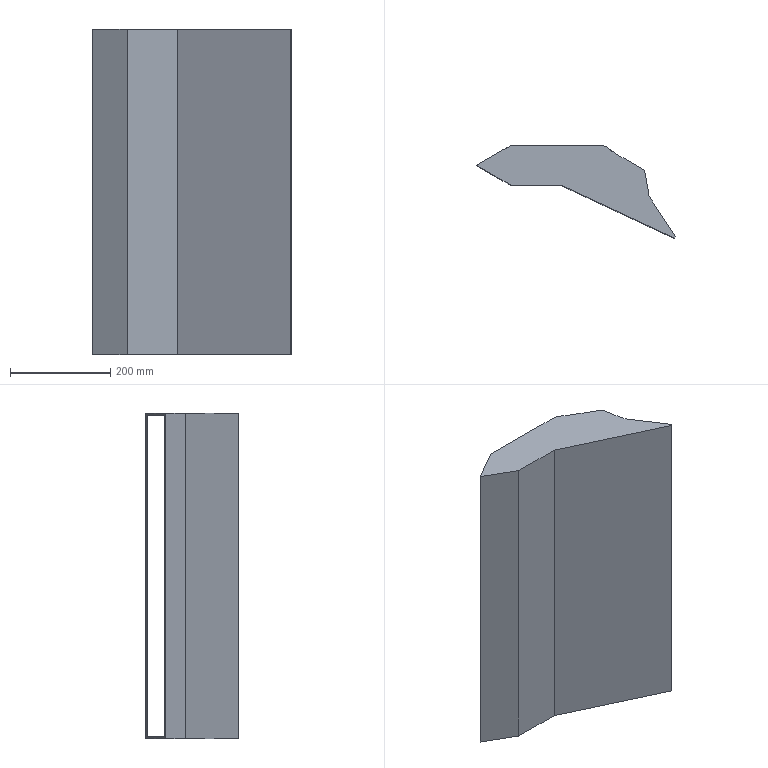Part | SolidWorks | features ICE 3, Extrusion 1, Shell 1 | 1 solid | 24 faces | box 397.808 x 185.717 x 650 mm | volume 1840134 mm3 | plane 23 | cylinder 1 | commonest cylinder face diameters 454 x1
STEP:
#1=CARTESIAN_POINT('',(-396.118,-217.427,-325.));
#2=VERTEX_POINT('',#1);
#3=CARTESIAN_POINT('',(-326.921,-177.476,-325.));
#4=VERTEX_POINT('',#3);
#5=CARTESIAN_POINT('',(-396.118,-217.427,-325.));
#6=DIRECTION('',(0.866,0.5,0.));
#7=VECTOR('',#6,1000.);
#8=LINE('',#5,#7);
#9=EDGE_CURVE('',#2,#4,#8,.T.);
#10=ORIENTED_EDGE('',*,*,#9,.F.);
#11=CARTESIAN_POINT('',(-396.118,-217.427,325.));
#12=VERTEX_POINT('',#11);
#13=CARTESIAN_POINT('',(-396.118,-217.427,-430.7));
#14=DIRECTION('',(0.,0.,1.));
#15=VECTOR('',#14,1000.);
#16=LINE('',#13,#15);
#17=EDGE_CURVE('',#2,#12,#16,.T.);
#18=ORIENTED_EDGE('',*,*,#17,.T.);
#19=CARTESIAN_POINT('',(-326.921,-177.476,325.));
#20=VERTEX_POINT('',#19);
#21=CARTESIAN_POINT('',(-396.118,-217.427,325.));
#22=DIRECTION('',(-0.866,-0.5,0.));
#23=VECTOR('',#22,1000.);
#24=LINE('',#21,#23);
#25=EDGE_CURVE('',#20,#12,#24,.T.);
#26=ORIENTED_EDGE('',*,*,#25,.F.);
#27=CARTESIAN_POINT('',(-326.921,-177.476,325.));
#28=DIRECTION('',(0.,0.,-1.));
#29=VECTOR('',#28,1000.);
#30=LINE('',#27,#29);
#31=EDGE_CURVE('',#20,#4,#30,.T.);
#32=ORIENTED_EDGE('',*,*,#31,.T.);
#33=EDGE_LOOP('',(#10,#18,#26,#32));
#34=FACE_OUTER_BOUND('',#33,.T.);
#35=CARTESIAN_POINT('',(-392.118,-215.118,-321.));
#36=VERTEX_POINT('',#35);
#37=CARTESIAN_POINT('',(-392.118,-215.118,321.));
#38=VERTEX_POINT('',#37);
#39=CARTESIAN_POINT('',(-392.118,-215.118,-430.7));
#40=DIRECTION('',(0.,0.,1.));
#41=VECTOR('',#40,1000.);
#42=LINE('',#39,#41);
#43=EDGE_CURVE('',#36,#38,#42,.T.);
#44=ORIENTED_EDGE('',*,*,#43,.F.);
#45=CARTESIAN_POINT('',(-333.849,-181.476,-321.));
#46=VERTEX_POINT('',#45);
#47=CARTESIAN_POINT('',(-396.118,-217.427,-321.));
#48=DIRECTION('',(0.866,0.5,0.));
#49=VECTOR('',#48,1000.);
#50=LINE('',#47,#49);
#51=EDGE_CURVE('',#36,#46,#50,.T.);
#52=ORIENTED_EDGE('',*,*,#51,.T.);
#53=CARTESIAN_POINT('',(-333.849,-181.476,321.));
#54=VERTEX_POINT('',#53);
#55=CARTESIAN_POINT('',(-333.849,-181.476,-430.7));
#56=DIRECTION('',(0.,0.,-1.));
#57=VECTOR('',#56,1000.);
#58=LINE('',#55,#57);
#59=EDGE_CURVE('',#54,#46,#58,.T.);
#60=ORIENTED_EDGE('',*,*,#59,.F.);
#61=CARTESIAN_POINT('',(-4.881,8.454,321.));
#62=DIRECTION('',(-0.866,-0.5,0.));
#63=VECTOR('',#62,1000.);
#64=LINE('',#61,#63);
#65=EDGE_CURVE('',#54,#38,#64,.T.);
#66=ORIENTED_EDGE('',*,*,#65,.T.);
#67=EDGE_LOOP('',(#44,#52,#60,#66));
#68=FACE_BOUND('',#67,.T.);
#69=CARTESIAN_POINT('',(-396.118,-217.427,-430.7));
#70=DIRECTION('',(-0.5,0.866,0.));
#71=DIRECTION('',(-0.866,-0.5,0.));
#72=AXIS2_PLACEMENT_3D('',#69,#70,#71);
#73=PLANE('',#72);
#74=ADVANCED_FACE('',(#34,#68),#73,.T.);
#75=CARTESIAN_POINT('',(1.69,-359.568,321.));
#76=VERTEX_POINT('',#75);
#77=CARTESIAN_POINT('',(1.69,-359.568,-321.));
#78=VERTEX_POINT('',#77);
#79=CARTESIAN_POINT('',(1.69,-359.568,325.));
#80=DIRECTION('',(0.,0.,-1.));
#81=VECTOR('',#80,1000.);
#82=LINE('',#79,#81);
#83=EDGE_CURVE('',#76,#78,#82,.T.);
#84=ORIENTED_EDGE('',*,*,#83,.T.);
#85=CARTESIAN_POINT('',(-226.034,-253.378,-321.));
#86=VERTEX_POINT('',#85);
#87=CARTESIAN_POINT('',(1.69,-359.568,-321.));
#88=DIRECTION('',(-0.9063,0.4226,0.));
#89=VECTOR('',#88,1000.);
#90=LINE('',#87,#89);
#91=EDGE_CURVE('',#78,#86,#90,.T.);
#92=ORIENTED_EDGE('',*,*,#91,.T.);
#93=CARTESIAN_POINT('',(-226.034,-253.378,321.));
#94=VERTEX_POINT('',#93);
#95=CARTESIAN_POINT('',(-226.034,-253.378,325.));
#96=DIRECTION('',(0.,0.,-1.));
#97=VECTOR('',#96,1000.);
#98=LINE('',#95,#97);
#99=EDGE_CURVE('',#94,#86,#98,.T.);
#100=ORIENTED_EDGE('',*,*,#99,.F.);
#101=CARTESIAN_POINT('',(-137.42,-294.699,321.));
#102=DIRECTION('',(0.9063,-0.4226,0.));
#103=VECTOR('',#102,1000.);
#104=LINE('',#101,#103);
#105=EDGE_CURVE('',#94,#76,#104,.T.);
#106=ORIENTED_EDGE('',*,*,#105,.T.);
#107=EDGE_LOOP('',(#84,#92,#100,#106));
#108=FACE_OUTER_BOUND('',#107,.T.);
#109=CARTESIAN_POINT('',(-137.42,-294.699,325.));
#110=DIRECTION('',(0.4226,0.9063,0.));
#111=DIRECTION('',(-0.9063,0.4226,0.));
#112=AXIS2_PLACEMENT_3D('',#109,#110,#111);
#113=PLANE('',#112);
#114=ADVANCED_FACE('',(#108),#113,.T.);
#115=CARTESIAN_POINT('',(-326.921,-253.378,-321.));
#116=VERTEX_POINT('',#115);
#117=CARTESIAN_POINT('',(-226.034,-253.378,-321.));
#118=DIRECTION('',(-1.,0.,0.));
#119=VECTOR('',#118,1000.);
#120=LINE('',#117,#119);
#121=EDGE_CURVE('',#86,#116,#120,.T.);
#122=ORIENTED_EDGE('',*,*,#121,.T.);
#123=CARTESIAN_POINT('',(-326.921,-253.378,321.));
#124=VERTEX_POINT('',#123);
#125=CARTESIAN_POINT('',(-326.921,-253.378,325.));
#126=DIRECTION('',(0.,0.,-1.));
#127=VECTOR('',#126,1000.);
#128=LINE('',#125,#127);
#129=EDGE_CURVE('',#124,#116,#128,.T.);
#130=ORIENTED_EDGE('',*,*,#129,.F.);
#131=CARTESIAN_POINT('',(0.,-253.378,321.));
#132=DIRECTION('',(-1.,0.,0.));
#133=VECTOR('',#132,1000.);
#134=LINE('',#131,#133);
#135=EDGE_CURVE('',#94,#124,#134,.T.);
#136=ORIENTED_EDGE('',*,*,#135,.F.);
#137=ORIENTED_EDGE('',*,*,#99,.T.);
#138=EDGE_LOOP('',(#122,#130,#136,#137));
#139=FACE_OUTER_BOUND('',#138,.T.);
#140=CARTESIAN_POINT('',(0.,-253.378,325.));
#141=DIRECTION('',(0.,-1.,0.));
#142=DIRECTION('',(0.,0.,-1.));
#143=AXIS2_PLACEMENT_3D('',#140,#141,#142);
#144=PLANE('',#143);
#145=ADVANCED_FACE('',(#139),#144,.F.);
#146=CARTESIAN_POINT('',(-136.365,-181.476,-321.));
#147=VERTEX_POINT('',#146);
#148=CARTESIAN_POINT('',(-326.921,-181.476,-321.));
#149=DIRECTION('',(1.,0.,0.));
#150=VECTOR('',#149,1000.);
#151=LINE('',#148,#150);
#152=EDGE_CURVE('',#46,#147,#151,.T.);
#153=ORIENTED_EDGE('',*,*,#152,.T.);
#154=CARTESIAN_POINT('',(-136.365,-181.476,321.));
#155=VERTEX_POINT('',#154);
#156=CARTESIAN_POINT('',(-136.365,-181.476,325.));
#157=DIRECTION('',(0.,0.,-1.));
#158=VECTOR('',#157,1000.);
#159=LINE('',#156,#158);
#160=EDGE_CURVE('',#155,#147,#159,.T.);
#161=ORIENTED_EDGE('',*,*,#160,.F.);
#162=CARTESIAN_POINT('',(0.,-181.476,321.));
#163=DIRECTION('',(1.,0.,0.));
#164=VECTOR('',#163,1000.);
#165=LINE('',#162,#164);
#166=EDGE_CURVE('',#54,#155,#165,.T.);
#167=ORIENTED_EDGE('',*,*,#166,.F.);
#168=ORIENTED_EDGE('',*,*,#59,.T.);
#169=EDGE_LOOP('',(#153,#161,#167,#168));
#170=FACE_OUTER_BOUND('',#169,.T.);
#171=CARTESIAN_POINT('',(0.,-181.476,325.));
#172=DIRECTION('',(0.,1.,0.));
#173=DIRECTION('',(0.,0.,1.));
#174=AXIS2_PLACEMENT_3D('',#171,#172,#173);
#175=PLANE('',#174);
#176=ADVANCED_FACE('',(#170),#175,.F.);
#177=CARTESIAN_POINT('',(1.69,-359.568,-325.));
#178=VERTEX_POINT('',#177);
#179=CARTESIAN_POINT('',(0.,-363.193,-325.));
#180=VERTEX_POINT('',#179);
#181=CARTESIAN_POINT('',(139.111,-64.868,-325.));
#182=DIRECTION('',(-0.4226,-0.9063,0.));
#183=VECTOR('',#182,1000.);
#184=LINE('',#181,#183);
#185=EDGE_CURVE('',#178,#180,#184,.T.);
#186=ORIENTED_EDGE('',*,*,#185,.F.);
#187=CARTESIAN_POINT('',(1.69,-359.568,-321.));
#188=DIRECTION('',(0.,0.,-1.));
#189=VECTOR('',#188,1000.);
#190=LINE('',#187,#189);
#191=EDGE_CURVE('',#78,#178,#190,.T.);
#192=ORIENTED_EDGE('',*,*,#191,.F.);
#193=ORIENTED_EDGE('',*,*,#83,.F.);
#194=CARTESIAN_POINT('',(1.69,-359.568,325.));
#195=VERTEX_POINT('',#194);
#196=CARTESIAN_POINT('',(1.69,-359.568,325.));
#197=DIRECTION('',(0.,0.,-1.));
#198=VECTOR('',#197,1000.);
#199=LINE('',#196,#198);
#200=EDGE_CURVE('',#195,#76,#199,.T.);
#201=ORIENTED_EDGE('',*,*,#200,.F.);
#202=CARTESIAN_POINT('',(0.,-363.193,325.));
#203=VERTEX_POINT('',#202);
#204=CARTESIAN_POINT('',(139.111,-64.868,325.));
#205=DIRECTION('',(-0.4226,-0.9063,0.));
#206=VECTOR('',#205,1000.);
#207=LINE('',#204,#206);
#208=EDGE_CURVE('',#195,#203,#207,.T.);
#209=ORIENTED_EDGE('',*,*,#208,.T.);
#210=CARTESIAN_POINT('',(0.,-363.193,325.));
#211=DIRECTION('',(0.,0.,-1.));
#212=VECTOR('',#211,1000.);
#213=LINE('',#210,#212);
#214=EDGE_CURVE('',#203,#180,#213,.T.);
#215=ORIENTED_EDGE('',*,*,#214,.T.);
#216=EDGE_LOOP('',(#186,#192,#193,#201,#209,#215));
#217=FACE_OUTER_BOUND('',#216,.T.);
#218=CARTESIAN_POINT('',(139.111,-64.868,325.));
#219=DIRECTION('',(0.9063,-0.4226,0.));
#220=DIRECTION('',(0.4226,0.9063,0.));
#221=AXIS2_PLACEMENT_3D('',#218,#219,#220);
#222=PLANE('',#221);
#223=ADVANCED_FACE('',(#217),#222,.T.);
#224=CARTESIAN_POINT('',(-226.921,-257.378,-325.));
#225=VERTEX_POINT('',#224);
#226=CARTESIAN_POINT('',(-326.921,-257.378,-325.));
#227=VERTEX_POINT('',#226);
#228=CARTESIAN_POINT('',(0.,-257.378,-325.));
#229=DIRECTION('',(-1.,0.,0.));
#230=VECTOR('',#229,1000.);
#231=LINE('',#228,#230);
#232=EDGE_CURVE('',#225,#227,#231,.T.);
#233=ORIENTED_EDGE('',*,*,#232,.F.);
#234=CARTESIAN_POINT('',(-226.921,-257.378,325.));
#235=VERTEX_POINT('',#234);
#236=CARTESIAN_POINT('',(-226.921,-257.378,325.));
#237=DIRECTION('',(0.,0.,-1.));
#238=VECTOR('',#237,1000.);
#239=LINE('',#236,#238);
#240=EDGE_CURVE('',#235,#225,#239,.T.);
#241=ORIENTED_EDGE('',*,*,#240,.F.);
#242=CARTESIAN_POINT('',(-326.921,-257.378,325.));
#243=VERTEX_POINT('',#242);
#244=CARTESIAN_POINT('',(0.,-257.378,325.));
#245=DIRECTION('',(-1.,0.,0.));
#246=VECTOR('',#245,1000.);
#247=LINE('',#244,#246);
#248=EDGE_CURVE('',#235,#243,#247,.T.);
#249=ORIENTED_EDGE('',*,*,#248,.T.);
#250=CARTESIAN_POINT('',(-326.921,-257.378,325.));
#251=DIRECTION('',(0.,0.,-1.));
#252=VECTOR('',#251,1000.);
#253=LINE('',#250,#252);
#254=EDGE_CURVE('',#243,#227,#253,.T.);
#255=ORIENTED_EDGE('',*,*,#254,.T.);
#256=EDGE_LOOP('',(#233,#241,#249,#255));
#257=FACE_OUTER_BOUND('',#256,.T.);
#258=CARTESIAN_POINT('',(0.,-257.378,325.));
#259=DIRECTION('',(0.,-1.,0.));
#260=DIRECTION('',(0.,0.,-1.));
#261=AXIS2_PLACEMENT_3D('',#258,#259,#260);
#262=PLANE('',#261);
#263=ADVANCED_FACE('',(#257),#262,.T.);
#264=CARTESIAN_POINT('',(-139.111,-298.324,-325.));
#265=DIRECTION('',(0.9063,-0.4226,0.));
#266=VECTOR('',#265,1000.);
#267=LINE('',#264,#266);
#268=EDGE_CURVE('',#225,#180,#267,.T.);
#269=ORIENTED_EDGE('',*,*,#268,.T.);
#270=ORIENTED_EDGE('',*,*,#214,.F.);
#271=CARTESIAN_POINT('',(-139.111,-298.324,325.));
#272=DIRECTION('',(0.9063,-0.4226,0.));
#273=VECTOR('',#272,1000.);
#274=LINE('',#271,#273);
#275=EDGE_CURVE('',#235,#203,#274,.T.);
#276=ORIENTED_EDGE('',*,*,#275,.F.);
#277=ORIENTED_EDGE('',*,*,#240,.T.);
#278=EDGE_LOOP('',(#269,#270,#276,#277));
#279=FACE_OUTER_BOUND('',#278,.T.);
#280=CARTESIAN_POINT('',(-139.111,-298.324,325.));
#281=DIRECTION('',(0.4226,0.9063,0.));
#282=DIRECTION('',(-0.9063,0.4226,0.));
#283=AXIS2_PLACEMENT_3D('',#280,#281,#282);
#284=PLANE('',#283);
#285=ADVANCED_FACE('',(#279),#284,.F.);
#286=ORIENTED_EDGE('',*,*,#208,.F.);
#287=CARTESIAN_POINT('',(-50.,-280.82,325.));
#288=VERTEX_POINT('',#287);
#289=CARTESIAN_POINT('',(-163.769,-107.499,325.));
#290=DIRECTION('',(0.5487,-0.836,0.));
#291=VECTOR('',#290,1000.);
#292=LINE('',#289,#291);
#293=EDGE_CURVE('',#288,#195,#292,.T.);
#294=ORIENTED_EDGE('',*,*,#293,.F.);
#295=CARTESIAN_POINT('',(-51.368,-277.061,325.));
#296=VERTEX_POINT('',#295);
#297=CARTESIAN_POINT('',(-134.405,-48.919,325.));
#298=DIRECTION('',(0.342,-0.9397,0.));
#299=VECTOR('',#298,1000.);
#300=LINE('',#297,#299);
#301=EDGE_CURVE('',#296,#288,#300,.T.);
#302=ORIENTED_EDGE('',*,*,#301,.F.);
#303=CARTESIAN_POINT('',(-60.,-227.476,325.));
#304=VERTEX_POINT('',#303);
#305=CARTESIAN_POINT('',(-96.67,-16.829,325.));
#306=DIRECTION('',(0.1715,-0.9852,0.));
#307=VECTOR('',#306,1000.);
#308=LINE('',#305,#307);
#309=EDGE_CURVE('',#304,#296,#308,.T.);
#310=ORIENTED_EDGE('',*,*,#309,.F.);
#311=CARTESIAN_POINT('',(-113.5,-196.588,325.));
#312=VERTEX_POINT('',#311);
#313=CARTESIAN_POINT('',(-113.5,-196.588,325.));
#314=DIRECTION('',(0.866,-0.5,0.));
#315=VECTOR('',#314,1000.);
#316=LINE('',#313,#315);
#317=EDGE_CURVE('',#312,#304,#316,.T.);
#318=ORIENTED_EDGE('',*,*,#317,.F.);
#319=CARTESIAN_POINT('',(-141.532,-177.476,325.));
#320=VERTEX_POINT('',#319);
#321=CARTESIAN_POINT('',(0.,0.,325.));
#322=DIRECTION('',(0.,0.,1.));
#323=DIRECTION('',(1.,0.,0.));
#324=AXIS2_PLACEMENT_3D('',#321,#322,#323);
#325=CIRCLE('',#324,227.);
#326=EDGE_CURVE('',#320,#312,#325,.T.);
#327=ORIENTED_EDGE('',*,*,#326,.F.);
#328=CARTESIAN_POINT('',(0.,-177.476,325.));
#329=DIRECTION('',(1.,0.,0.));
#330=VECTOR('',#329,1000.);
#331=LINE('',#328,#330);
#332=EDGE_CURVE('',#20,#320,#331,.T.);
#333=ORIENTED_EDGE('',*,*,#332,.F.);
#334=ORIENTED_EDGE('',*,*,#25,.T.);
#335=CARTESIAN_POINT('',(-326.921,-257.378,325.));
#336=DIRECTION('',(0.866,-0.5,0.));
#337=VECTOR('',#336,1000.);
#338=LINE('',#335,#337);
#339=EDGE_CURVE('',#12,#243,#338,.T.);
#340=ORIENTED_EDGE('',*,*,#339,.T.);
#341=ORIENTED_EDGE('',*,*,#248,.F.);
#342=ORIENTED_EDGE('',*,*,#275,.T.);
#343=EDGE_LOOP('',(#286,#294,#302,#310,#318,#327,#333,#334,#340,#341,#342));
#344=FACE_OUTER_BOUND('',#343,.T.);
#345=CARTESIAN_POINT('',(0.,0.,325.));
#346=DIRECTION('',(0.,0.,1.));
#347=DIRECTION('',(1.,0.,0.));
#348=AXIS2_PLACEMENT_3D('',#345,#346,#347);
#349=PLANE('',#348);
#350=ADVANCED_FACE('',(#344),#349,.T.);
#351=ORIENTED_EDGE('',*,*,#232,.T.);
#352=CARTESIAN_POINT('',(-326.921,-257.378,-325.));
#353=DIRECTION('',(-0.866,0.5,0.));
#354=VECTOR('',#353,1000.);
#355=LINE('',#352,#354);
#356=EDGE_CURVE('',#227,#2,#355,.T.);
#357=ORIENTED_EDGE('',*,*,#356,.T.);
#358=ORIENTED_EDGE('',*,*,#9,.T.);
#359=CARTESIAN_POINT('',(-141.532,-177.476,-325.));
#360=VERTEX_POINT('',#359);
#361=CARTESIAN_POINT('',(0.,-177.476,-325.));
#362=DIRECTION('',(1.,0.,0.));
#363=VECTOR('',#362,1000.);
#364=LINE('',#361,#363);
#365=EDGE_CURVE('',#4,#360,#364,.T.);
#366=ORIENTED_EDGE('',*,*,#365,.T.);
#367=CARTESIAN_POINT('',(-113.5,-196.588,-325.));
#368=VERTEX_POINT('',#367);
#369=CARTESIAN_POINT('',(0.,0.,-325.));
#370=DIRECTION('',(0.,0.,1.));
#371=DIRECTION('',(1.,0.,0.));
#372=AXIS2_PLACEMENT_3D('',#369,#370,#371);
#373=CIRCLE('',#372,227.);
#374=EDGE_CURVE('',#360,#368,#373,.T.);
#375=ORIENTED_EDGE('',*,*,#374,.T.);
#376=CARTESIAN_POINT('',(-60.,-227.476,-325.));
#377=VERTEX_POINT('',#376);
#378=CARTESIAN_POINT('',(-113.5,-196.588,-325.));
#379=DIRECTION('',(0.866,-0.5,0.));
#380=VECTOR('',#379,1000.);
#381=LINE('',#378,#380);
#382=EDGE_CURVE('',#368,#377,#381,.T.);
#383=ORIENTED_EDGE('',*,*,#382,.T.);
#384=CARTESIAN_POINT('',(-51.368,-277.061,-325.));
#385=VERTEX_POINT('',#384);
#386=CARTESIAN_POINT('',(-60.,-227.476,-325.));
#387=DIRECTION('',(0.1715,-0.9852,0.));
#388=VECTOR('',#387,1000.);
#389=LINE('',#386,#388);
#390=EDGE_CURVE('',#377,#385,#389,.T.);
#391=ORIENTED_EDGE('',*,*,#390,.T.);
#392=CARTESIAN_POINT('',(-50.,-280.82,-325.));
#393=VERTEX_POINT('',#392);
#394=CARTESIAN_POINT('',(-51.368,-277.061,-325.));
#395=DIRECTION('',(0.342,-0.9397,0.));
#396=VECTOR('',#395,1000.);
#397=LINE('',#394,#396);
#398=EDGE_CURVE('',#385,#393,#397,.T.);
#399=ORIENTED_EDGE('',*,*,#398,.T.);
#400=CARTESIAN_POINT('',(-50.,-280.82,-325.));
#401=DIRECTION('',(0.5487,-0.836,0.));
#402=VECTOR('',#401,1000.);
#403=LINE('',#400,#402);
#404=EDGE_CURVE('',#393,#178,#403,.T.);
#405=ORIENTED_EDGE('',*,*,#404,.T.);
#406=ORIENTED_EDGE('',*,*,#185,.T.);
#407=ORIENTED_EDGE('',*,*,#268,.F.);
#408=EDGE_LOOP('',(#351,#357,#358,#366,#375,#383,#391,#399,#405,#406,#407));
#409=FACE_OUTER_BOUND('',#408,.T.);
#410=CARTESIAN_POINT('',(0.,0.,-325.));
#411=DIRECTION('',(0.,0.,1.));
#412=DIRECTION('',(1.,0.,0.));
#413=AXIS2_PLACEMENT_3D('',#410,#411,#412);
#414=PLANE('',#413);
#415=ADVANCED_FACE('',(#409),#414,.F.);
#416=ORIENTED_EDGE('',*,*,#326,.T.);
#417=CARTESIAN_POINT('',(-113.5,-196.588,321.));
#418=VERTEX_POINT('',#417);
#419=CARTESIAN_POINT('',(-113.5,-196.588,321.));
#420=DIRECTION('',(0.,0.,1.));
#421=VECTOR('',#420,1000.);
#422=LINE('',#419,#421);
#423=EDGE_CURVE('',#418,#312,#422,.T.);
#424=ORIENTED_EDGE('',*,*,#423,.F.);
#425=CARTESIAN_POINT('',(0.,0.,321.));
#426=DIRECTION('',(0.,0.,1.));
#427=DIRECTION('',(1.,0.,0.));
#428=AXIS2_PLACEMENT_3D('',#425,#426,#427);
#429=CIRCLE('',#428,227.);
#430=EDGE_CURVE('',#155,#418,#429,.T.);
#431=ORIENTED_EDGE('',*,*,#430,.F.);
#432=ORIENTED_EDGE('',*,*,#160,.T.);
#433=CARTESIAN_POINT('',(-113.5,-196.588,-321.));
#434=VERTEX_POINT('',#433);
#435=CARTESIAN_POINT('',(0.,0.,-321.));
#436=DIRECTION('',(0.,0.,1.));
#437=DIRECTION('',(-1.,0.,0.));
#438=AXIS2_PLACEMENT_3D('',#435,#436,#437);
#439=CIRCLE('',#438,227.);
#440=EDGE_CURVE('',#147,#434,#439,.T.);
#441=ORIENTED_EDGE('',*,*,#440,.T.);
#442=CARTESIAN_POINT('',(-113.5,-196.588,-321.));
#443=DIRECTION('',(0.,0.,-1.));
#444=VECTOR('',#443,1000.);
#445=LINE('',#442,#444);
#446=EDGE_CURVE('',#434,#368,#445,.T.);
#447=ORIENTED_EDGE('',*,*,#446,.T.);
#448=ORIENTED_EDGE('',*,*,#374,.F.);
#449=CARTESIAN_POINT('',(-141.532,-177.476,325.));
#450=DIRECTION('',(0.,0.,-1.));
#451=VECTOR('',#450,1000.);
#452=LINE('',#449,#451);
#453=EDGE_CURVE('',#320,#360,#452,.T.);
#454=ORIENTED_EDGE('',*,*,#453,.F.);
#455=EDGE_LOOP('',(#416,#424,#431,#432,#441,#447,#448,#454));
#456=FACE_OUTER_BOUND('',#455,.T.);
#457=CARTESIAN_POINT('',(0.,0.,321.));
#458=DIRECTION('',(0.,0.,1.));
#459=DIRECTION('',(1.,0.,0.));
#460=AXIS2_PLACEMENT_3D('',#457,#458,#459);
#461=CYLINDRICAL_SURFACE('',#460,227.);
#462=ADVANCED_FACE('',(#456),#461,.F.);
#463=ORIENTED_EDGE('',*,*,#317,.T.);
#464=CARTESIAN_POINT('',(-60.,-227.476,321.));
#465=VERTEX_POINT('',#464);
#466=CARTESIAN_POINT('',(-60.,-227.476,321.));
#467=DIRECTION('',(0.,0.,1.));
#468=VECTOR('',#467,1000.);
#469=LINE('',#466,#468);
#470=EDGE_CURVE('',#465,#304,#469,.T.);
#471=ORIENTED_EDGE('',*,*,#470,.F.);
#472=CARTESIAN_POINT('',(-113.5,-196.588,321.));
#473=DIRECTION('',(0.866,-0.5,0.));
#474=VECTOR('',#473,1000.);
#475=LINE('',#472,#474);
#476=EDGE_CURVE('',#418,#465,#475,.T.);
#477=ORIENTED_EDGE('',*,*,#476,.F.);
#478=ORIENTED_EDGE('',*,*,#423,.T.);
#479=EDGE_LOOP('',(#463,#471,#477,#478));
#480=FACE_OUTER_BOUND('',#479,.T.);
#481=CARTESIAN_POINT('',(-113.5,-196.588,321.));
#482=DIRECTION('',(-0.5,-0.866,0.));
#483=DIRECTION('',(0.866,-0.5,0.));
#484=AXIS2_PLACEMENT_3D('',#481,#482,#483);
#485=PLANE('',#484);
#486=ADVANCED_FACE('',(#480),#485,.F.);
#487=ORIENTED_EDGE('',*,*,#309,.T.);
#488=CARTESIAN_POINT('',(-51.368,-277.061,321.));
#489=VERTEX_POINT('',#488);
#490=CARTESIAN_POINT('',(-51.368,-277.061,321.));
#491=DIRECTION('',(0.,0.,1.));
#492=VECTOR('',#491,1000.);
#493=LINE('',#490,#492);
#494=EDGE_CURVE('',#489,#296,#493,.T.);
#495=ORIENTED_EDGE('',*,*,#494,.F.);
#496=CARTESIAN_POINT('',(-96.67,-16.829,321.));
#497=DIRECTION('',(0.1715,-0.9852,0.));
#498=VECTOR('',#497,1000.);
#499=LINE('',#496,#498);
#500=EDGE_CURVE('',#465,#489,#499,.T.);
#501=ORIENTED_EDGE('',*,*,#500,.F.);
#502=ORIENTED_EDGE('',*,*,#470,.T.);
#503=EDGE_LOOP('',(#487,#495,#501,#502));
#504=FACE_OUTER_BOUND('',#503,.T.);
#505=CARTESIAN_POINT('',(-96.67,-16.829,321.));
#506=DIRECTION('',(-0.9852,-0.1715,0.));
#507=DIRECTION('',(0.1715,-0.9852,0.));
#508=AXIS2_PLACEMENT_3D('',#505,#506,#507);
#509=PLANE('',#508);
#510=ADVANCED_FACE('',(#504),#509,.F.);
#511=ORIENTED_EDGE('',*,*,#301,.T.);
#512=CARTESIAN_POINT('',(-50.,-280.82,321.));
#513=VERTEX_POINT('',#512);
#514=CARTESIAN_POINT('',(-50.,-280.82,321.));
#515=DIRECTION('',(0.,0.,1.));
#516=VECTOR('',#515,1000.);
#517=LINE('',#514,#516);
#518=EDGE_CURVE('',#513,#288,#517,.T.);
#519=ORIENTED_EDGE('',*,*,#518,.F.);
#520=CARTESIAN_POINT('',(-134.405,-48.919,321.));
#521=DIRECTION('',(0.342,-0.9397,0.));
#522=VECTOR('',#521,1000.);
#523=LINE('',#520,#522);
#524=EDGE_CURVE('',#489,#513,#523,.T.);
#525=ORIENTED_EDGE('',*,*,#524,.F.);
#526=ORIENTED_EDGE('',*,*,#494,.T.);
#527=EDGE_LOOP('',(#511,#519,#525,#526));
#528=FACE_OUTER_BOUND('',#527,.T.);
#529=CARTESIAN_POINT('',(-134.405,-48.919,321.));
#530=DIRECTION('',(-0.9397,-0.342,0.));
#531=DIRECTION('',(0.342,-0.9397,0.));
#532=AXIS2_PLACEMENT_3D('',#529,#530,#531);
#533=PLANE('',#532);
#534=ADVANCED_FACE('',(#528),#533,.F.);
#535=ORIENTED_EDGE('',*,*,#293,.T.);
#536=ORIENTED_EDGE('',*,*,#200,.T.);
#537=CARTESIAN_POINT('',(-163.769,-107.499,321.));
#538=DIRECTION('',(0.5487,-0.836,0.));
#539=VECTOR('',#538,1000.);
#540=LINE('',#537,#539);
#541=EDGE_CURVE('',#513,#76,#540,.T.);
#542=ORIENTED_EDGE('',*,*,#541,.F.);
#543=ORIENTED_EDGE('',*,*,#518,.T.);
#544=EDGE_LOOP('',(#535,#536,#542,#543));
#545=FACE_OUTER_BOUND('',#544,.T.);
#546=CARTESIAN_POINT('',(-163.769,-107.499,321.));
#547=DIRECTION('',(-0.836,-0.5487,0.));
#548=DIRECTION('',(0.5487,-0.836,0.));
#549=AXIS2_PLACEMENT_3D('',#546,#547,#548);
#550=PLANE('',#549);
#551=ADVANCED_FACE('',(#545),#550,.F.);
#552=ORIENTED_EDGE('',*,*,#430,.T.);
#553=ORIENTED_EDGE('',*,*,#476,.T.);
#554=ORIENTED_EDGE('',*,*,#500,.T.);
#555=ORIENTED_EDGE('',*,*,#524,.T.);
#556=ORIENTED_EDGE('',*,*,#541,.T.);
#557=ORIENTED_EDGE('',*,*,#105,.F.);
#558=ORIENTED_EDGE('',*,*,#135,.T.);
#559=CARTESIAN_POINT('',(-326.921,-252.759,321.));
#560=VERTEX_POINT('',#559);
#561=CARTESIAN_POINT('',(-326.921,0.,321.));
#562=DIRECTION('',(0.,1.,0.));
#563=VECTOR('',#562,1000.);
#564=LINE('',#561,#563);
#565=EDGE_CURVE('',#124,#560,#564,.T.);
#566=ORIENTED_EDGE('',*,*,#565,.T.);
#567=CARTESIAN_POINT('',(-191.178,-331.13,321.));
#568=DIRECTION('',(0.866,-0.5,0.));
#569=VECTOR('',#568,1000.);
#570=LINE('',#567,#569);
#571=EDGE_CURVE('',#38,#560,#570,.T.);
#572=ORIENTED_EDGE('',*,*,#571,.F.);
#573=ORIENTED_EDGE('',*,*,#65,.F.);
#574=ORIENTED_EDGE('',*,*,#166,.T.);
#575=EDGE_LOOP('',(#552,#553,#554,#555,#556,#557,#558,#566,#572,#573,#574));
#576=FACE_OUTER_BOUND('',#575,.T.);
#577=CARTESIAN_POINT('',(0.,0.,321.));
#578=DIRECTION('',(0.,0.,1.));
#579=DIRECTION('',(1.,0.,0.));
#580=AXIS2_PLACEMENT_3D('',#577,#578,#579);
#581=PLANE('',#580);
#582=ADVANCED_FACE('',(#576),#581,.F.);
#583=ORIENTED_EDGE('',*,*,#365,.F.);
#584=ORIENTED_EDGE('',*,*,#31,.F.);
#585=ORIENTED_EDGE('',*,*,#332,.T.);
#586=ORIENTED_EDGE('',*,*,#453,.T.);
#587=EDGE_LOOP('',(#583,#584,#585,#586));
#588=FACE_OUTER_BOUND('',#587,.T.);
#589=CARTESIAN_POINT('',(0.,-177.476,325.));
#590=DIRECTION('',(0.,1.,0.));
#591=DIRECTION('',(0.,0.,1.));
#592=AXIS2_PLACEMENT_3D('',#589,#590,#591);
#593=PLANE('',#592);
#594=ADVANCED_FACE('',(#588),#593,.T.);
#595=ORIENTED_EDGE('',*,*,#404,.F.);
#596=CARTESIAN_POINT('',(-50.,-280.82,-321.));
#597=VERTEX_POINT('',#596);
#598=CARTESIAN_POINT('',(-50.,-280.82,-321.));
#599=DIRECTION('',(0.,0.,-1.));
#600=VECTOR('',#599,1000.);
#601=LINE('',#598,#600);
#602=EDGE_CURVE('',#597,#393,#601,.T.);
#603=ORIENTED_EDGE('',*,*,#602,.F.);
#604=CARTESIAN_POINT('',(-50.,-280.82,-321.));
#605=DIRECTION('',(0.5487,-0.836,0.));
#606=VECTOR('',#605,1000.);
#607=LINE('',#604,#606);
#608=EDGE_CURVE('',#597,#78,#607,.T.);
#609=ORIENTED_EDGE('',*,*,#608,.T.);
#610=ORIENTED_EDGE('',*,*,#191,.T.);
#611=EDGE_LOOP('',(#595,#603,#609,#610));
#612=FACE_OUTER_BOUND('',#611,.T.);
#613=CARTESIAN_POINT('',(-50.,-280.82,-321.));
#614=DIRECTION('',(0.836,0.5487,0.));
#615=DIRECTION('',(-0.5487,0.836,0.));
#616=AXIS2_PLACEMENT_3D('',#613,#614,#615);
#617=PLANE('',#616);
#618=ADVANCED_FACE('',(#612),#617,.T.);
#619=ORIENTED_EDGE('',*,*,#398,.F.);
#620=CARTESIAN_POINT('',(-51.368,-277.061,-321.));
#621=VERTEX_POINT('',#620);
#622=CARTESIAN_POINT('',(-51.368,-277.061,-321.));
#623=DIRECTION('',(0.,0.,-1.));
#624=VECTOR('',#623,1000.);
#625=LINE('',#622,#624);
#626=EDGE_CURVE('',#621,#385,#625,.T.);
#627=ORIENTED_EDGE('',*,*,#626,.F.);
#628=CARTESIAN_POINT('',(-51.368,-277.061,-321.));
#629=DIRECTION('',(0.342,-0.9397,0.));
#630=VECTOR('',#629,1000.);
#631=LINE('',#628,#630);
#632=EDGE_CURVE('',#621,#597,#631,.T.);
#633=ORIENTED_EDGE('',*,*,#632,.T.);
#634=ORIENTED_EDGE('',*,*,#602,.T.);
#635=EDGE_LOOP('',(#619,#627,#633,#634));
#636=FACE_OUTER_BOUND('',#635,.T.);
#637=CARTESIAN_POINT('',(-51.368,-277.061,-321.));
#638=DIRECTION('',(0.9397,0.342,0.));
#639=DIRECTION('',(-0.342,0.9397,0.));
#640=AXIS2_PLACEMENT_3D('',#637,#638,#639);
#641=PLANE('',#640);
#642=ADVANCED_FACE('',(#636),#641,.T.);
#643=ORIENTED_EDGE('',*,*,#390,.F.);
#644=CARTESIAN_POINT('',(-60.,-227.476,-321.));
#645=VERTEX_POINT('',#644);
#646=CARTESIAN_POINT('',(-60.,-227.476,-321.));
#647=DIRECTION('',(0.,0.,-1.));
#648=VECTOR('',#647,1000.);
#649=LINE('',#646,#648);
#650=EDGE_CURVE('',#645,#377,#649,.T.);
#651=ORIENTED_EDGE('',*,*,#650,.F.);
#652=CARTESIAN_POINT('',(-60.,-227.476,-321.));
#653=DIRECTION('',(0.1715,-0.9852,0.));
#654=VECTOR('',#653,1000.);
#655=LINE('',#652,#654);
#656=EDGE_CURVE('',#645,#621,#655,.T.);
#657=ORIENTED_EDGE('',*,*,#656,.T.);
#658=ORIENTED_EDGE('',*,*,#626,.T.);
#659=EDGE_LOOP('',(#643,#651,#657,#658));
#660=FACE_OUTER_BOUND('',#659,.T.);
#661=CARTESIAN_POINT('',(-60.,-227.476,-321.));
#662=DIRECTION('',(0.9852,0.1715,0.));
#663=DIRECTION('',(-0.1715,0.9852,0.));
#664=AXIS2_PLACEMENT_3D('',#661,#662,#663);
#665=PLANE('',#664);
#666=ADVANCED_FACE('',(#660),#665,.T.);
#667=ORIENTED_EDGE('',*,*,#382,.F.);
#668=ORIENTED_EDGE('',*,*,#446,.F.);
#669=CARTESIAN_POINT('',(-113.5,-196.588,-321.));
#670=DIRECTION('',(0.866,-0.5,0.));
#671=VECTOR('',#670,1000.);
#672=LINE('',#669,#671);
#673=EDGE_CURVE('',#434,#645,#672,.T.);
#674=ORIENTED_EDGE('',*,*,#673,.T.);
#675=ORIENTED_EDGE('',*,*,#650,.T.);
#676=EDGE_LOOP('',(#667,#668,#674,#675));
#677=FACE_OUTER_BOUND('',#676,.T.);
#678=CARTESIAN_POINT('',(-113.5,-196.588,-321.));
#679=DIRECTION('',(0.5,0.866,0.));
#680=DIRECTION('',(-0.866,0.5,0.));
#681=AXIS2_PLACEMENT_3D('',#678,#679,#680);
#682=PLANE('',#681);
#683=ADVANCED_FACE('',(#677),#682,.T.);
#684=ORIENTED_EDGE('',*,*,#440,.F.);
#685=ORIENTED_EDGE('',*,*,#152,.F.);
#686=ORIENTED_EDGE('',*,*,#51,.F.);
#687=CARTESIAN_POINT('',(-326.921,-252.759,-321.));
#688=VERTEX_POINT('',#687);
#689=CARTESIAN_POINT('',(-324.921,-253.914,-321.));
#690=DIRECTION('',(-0.866,0.5,0.));
#691=VECTOR('',#690,1000.);
#692=LINE('',#689,#691);
#693=EDGE_CURVE('',#688,#36,#692,.T.);
#694=ORIENTED_EDGE('',*,*,#693,.F.);
#695=CARTESIAN_POINT('',(-326.921,-253.378,-321.));
#696=DIRECTION('',(0.,1.,0.));
#697=VECTOR('',#696,1000.);
#698=LINE('',#695,#697);
#699=EDGE_CURVE('',#116,#688,#698,.T.);
#700=ORIENTED_EDGE('',*,*,#699,.F.);
#701=ORIENTED_EDGE('',*,*,#121,.F.);
#702=ORIENTED_EDGE('',*,*,#91,.F.);
#703=ORIENTED_EDGE('',*,*,#608,.F.);
#704=ORIENTED_EDGE('',*,*,#632,.F.);
#705=ORIENTED_EDGE('',*,*,#656,.F.);
#706=ORIENTED_EDGE('',*,*,#673,.F.);
#707=EDGE_LOOP('',(#684,#685,#686,#694,#700,#701,#702,#703,#704,#705,#706));
#708=FACE_OUTER_BOUND('',#707,.T.);
#709=CARTESIAN_POINT('',(0.,0.,-321.));
#710=DIRECTION('',(0.,0.,-1.));
#711=DIRECTION('',(-1.,0.,0.));
#712=AXIS2_PLACEMENT_3D('',#709,#710,#711);
#713=PLANE('',#712);
#714=ADVANCED_FACE('',(#708),#713,.F.);
#715=CARTESIAN_POINT('',(-326.921,-252.759,-430.7));
#716=DIRECTION('',(0.,0.,-1.));
#717=VECTOR('',#716,1000.);
#718=LINE('',#715,#717);
#719=EDGE_CURVE('',#560,#688,#718,.T.);
#720=ORIENTED_EDGE('',*,*,#719,.F.);
#721=ORIENTED_EDGE('',*,*,#565,.F.);
#722=ORIENTED_EDGE('',*,*,#129,.T.);
#723=ORIENTED_EDGE('',*,*,#699,.T.);
#724=EDGE_LOOP('',(#720,#721,#722,#723));
#725=FACE_OUTER_BOUND('',#724,.T.);
#726=CARTESIAN_POINT('',(-326.921,-177.476,-430.7));
#727=DIRECTION('',(1.,0.,0.));
#728=DIRECTION('',(0.,0.,-1.));
#729=AXIS2_PLACEMENT_3D('',#726,#727,#728);
#730=PLANE('',#729);
#731=ADVANCED_FACE('',(#725),#730,.T.);
#732=ORIENTED_EDGE('',*,*,#356,.F.);
#733=ORIENTED_EDGE('',*,*,#254,.F.);
#734=ORIENTED_EDGE('',*,*,#339,.F.);
#735=ORIENTED_EDGE('',*,*,#17,.F.);
#736=EDGE_LOOP('',(#732,#733,#734,#735));
#737=FACE_OUTER_BOUND('',#736,.T.);
#738=CARTESIAN_POINT('',(-326.921,-257.378,-430.7));
#739=DIRECTION('',(-0.5,-0.866,0.));
#740=DIRECTION('',(0.866,-0.5,0.));
#741=AXIS2_PLACEMENT_3D('',#738,#739,#740);
#742=PLANE('',#741);
#743=ADVANCED_FACE('',(#737),#742,.T.);
#744=ORIENTED_EDGE('',*,*,#719,.T.);
#745=ORIENTED_EDGE('',*,*,#693,.T.);
#746=ORIENTED_EDGE('',*,*,#43,.T.);
#747=ORIENTED_EDGE('',*,*,#571,.T.);
#748=EDGE_LOOP('',(#744,#745,#746,#747));
#749=FACE_OUTER_BOUND('',#748,.T.);
#750=CARTESIAN_POINT('',(-324.921,-253.914,-430.7));
#751=DIRECTION('',(-0.5,-0.866,0.));
#752=DIRECTION('',(0.866,-0.5,0.));
#753=AXIS2_PLACEMENT_3D('',#750,#751,#752);
#754=PLANE('',#753);
#755=ADVANCED_FACE('',(#749),#754,.F.);
#756=CLOSED_SHELL('',(#74,#114,#145,#176,#223,#263,#285,#350,#415,#462,#486,#510,#534,#551,#582,#594,#618,#642,#666,#683,#714,#731,#743,#755));
#757=MANIFOLD_SOLID_BREP('',#756);
#758=CARTESIAN_POINT('',(0.,0.,0.));
#759=DIRECTION('',(0.,0.,1.));
#760=DIRECTION('',(1.,0.,0.));
#761=AXIS2_PLACEMENT_3D('',#758,#759,#760);
#762=(LENGTH_UNIT()NAMED_UNIT(*)SI_UNIT(.MILLI.,.METRE.));
#763=UNCERTAINTY_MEASURE_WITH_UNIT(LENGTH_MEASURE(0.00001),#762,'','');
#764=(NAMED_UNIT(*)PLANE_ANGLE_UNIT()SI_UNIT($,.RADIAN.));
#765=(NAMED_UNIT(*)SI_UNIT($,.STERADIAN.)SOLID_ANGLE_UNIT());
#766=(GEOMETRIC_REPRESENTATION_CONTEXT(3)GLOBAL_UNCERTAINTY_ASSIGNED_CONTEXT((#763))GLOBAL_UNIT_ASSIGNED_CONTEXT((#762,#764,#765))REPRESENTATION_CONTEXT('',''));
#767=ADVANCED_BREP_SHAPE_REPRESENTATION('',(#757,#761),#766);